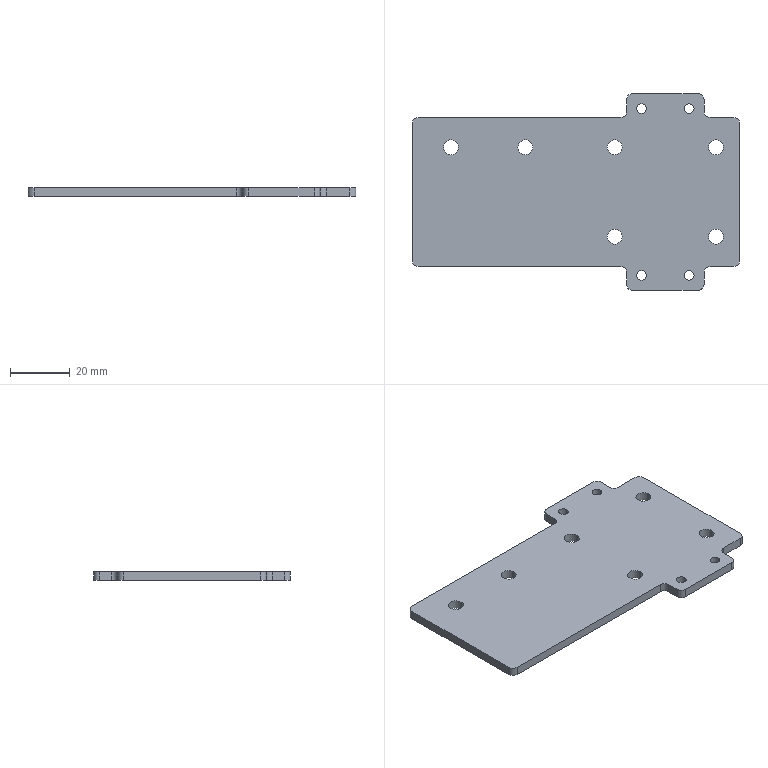Part | SolidWorks | features BaseBody 1 | 1 solid | 46 faces | box 110 x 66 x 3 mm | volume 17285 mm3 | cylinder 32 | plane 14 | commonest cylinder face diameters 4 x12 5 x12 3.24 x8
STEP:
#1=CARTESIAN_POINT('',(20.38,-28.,3.));
#2=VERTEX_POINT('',#1);
#3=CARTESIAN_POINT('',(23.62,-28.,3.));
#4=VERTEX_POINT('',#3);
#5=CARTESIAN_POINT('',(22.,-28.,3.));
#6=DIRECTION('',(0.,0.,1.));
#7=DIRECTION('',(-1.,0.,0.));
#8=AXIS2_PLACEMENT_3D('',#5,#6,#7);
#9=CIRCLE('',#8,1.62);
#10=EDGE_CURVE('',#2,#4,#9,.T.);
#11=ORIENTED_EDGE('',*,*,#10,.T.);
#12=CARTESIAN_POINT('',(23.62,-28.,0.));
#13=VERTEX_POINT('',#12);
#14=CARTESIAN_POINT('',(23.62,-28.,3.));
#15=DIRECTION('',(0.,0.,-1.));
#16=VECTOR('',#15,1000.);
#17=LINE('',#14,#16);
#18=EDGE_CURVE('',#4,#13,#17,.T.);
#19=ORIENTED_EDGE('',*,*,#18,.T.);
#20=CARTESIAN_POINT('',(20.38,-28.,0.));
#21=VERTEX_POINT('',#20);
#22=CARTESIAN_POINT('',(22.,-28.,0.));
#23=DIRECTION('',(0.,0.,1.));
#24=DIRECTION('',(-1.,0.,0.));
#25=AXIS2_PLACEMENT_3D('',#22,#23,#24);
#26=CIRCLE('',#25,1.62);
#27=EDGE_CURVE('',#21,#13,#26,.T.);
#28=ORIENTED_EDGE('',*,*,#27,.F.);
#29=CARTESIAN_POINT('',(20.38,-28.,3.));
#30=DIRECTION('',(0.,0.,-1.));
#31=VECTOR('',#30,1000.);
#32=LINE('',#29,#31);
#33=EDGE_CURVE('',#2,#21,#32,.T.);
#34=ORIENTED_EDGE('',*,*,#33,.F.);
#35=EDGE_LOOP('',(#11,#19,#28,#34));
#36=FACE_OUTER_BOUND('',#35,.T.);
#37=CARTESIAN_POINT('',(22.,-28.,3.));
#38=DIRECTION('',(0.,0.,-1.));
#39=DIRECTION('',(-1.,0.,0.));
#40=AXIS2_PLACEMENT_3D('',#37,#38,#39);
#41=CYLINDRICAL_SURFACE('',#40,1.62);
#42=ADVANCED_FACE('',(#36),#41,.F.);
#43=CARTESIAN_POINT('',(36.38,-28.,3.));
#44=VERTEX_POINT('',#43);
#45=CARTESIAN_POINT('',(39.62,-28.,3.));
#46=VERTEX_POINT('',#45);
#47=CARTESIAN_POINT('',(38.,-28.,3.));
#48=DIRECTION('',(0.,0.,1.));
#49=DIRECTION('',(-1.,0.,0.));
#50=AXIS2_PLACEMENT_3D('',#47,#48,#49);
#51=CIRCLE('',#50,1.62);
#52=EDGE_CURVE('',#44,#46,#51,.T.);
#53=ORIENTED_EDGE('',*,*,#52,.T.);
#54=CARTESIAN_POINT('',(39.62,-28.,0.));
#55=VERTEX_POINT('',#54);
#56=CARTESIAN_POINT('',(39.62,-28.,3.));
#57=DIRECTION('',(0.,0.,-1.));
#58=VECTOR('',#57,1000.);
#59=LINE('',#56,#58);
#60=EDGE_CURVE('',#46,#55,#59,.T.);
#61=ORIENTED_EDGE('',*,*,#60,.T.);
#62=CARTESIAN_POINT('',(36.38,-28.,0.));
#63=VERTEX_POINT('',#62);
#64=CARTESIAN_POINT('',(38.,-28.,0.));
#65=DIRECTION('',(0.,0.,1.));
#66=DIRECTION('',(-1.,0.,0.));
#67=AXIS2_PLACEMENT_3D('',#64,#65,#66);
#68=CIRCLE('',#67,1.62);
#69=EDGE_CURVE('',#63,#55,#68,.T.);
#70=ORIENTED_EDGE('',*,*,#69,.F.);
#71=CARTESIAN_POINT('',(36.38,-28.,3.));
#72=DIRECTION('',(0.,0.,-1.));
#73=VECTOR('',#72,1000.);
#74=LINE('',#71,#73);
#75=EDGE_CURVE('',#44,#63,#74,.T.);
#76=ORIENTED_EDGE('',*,*,#75,.F.);
#77=EDGE_LOOP('',(#53,#61,#70,#76));
#78=FACE_OUTER_BOUND('',#77,.T.);
#79=CARTESIAN_POINT('',(38.,-28.,3.));
#80=DIRECTION('',(0.,0.,-1.));
#81=DIRECTION('',(-1.,0.,0.));
#82=AXIS2_PLACEMENT_3D('',#79,#80,#81);
#83=CYLINDRICAL_SURFACE('',#82,1.62);
#84=ADVANCED_FACE('',(#78),#83,.F.);
#85=CARTESIAN_POINT('',(36.38,28.,3.));
#86=VERTEX_POINT('',#85);
#87=CARTESIAN_POINT('',(39.62,28.,3.));
#88=VERTEX_POINT('',#87);
#89=CARTESIAN_POINT('',(38.,28.,3.));
#90=DIRECTION('',(0.,0.,1.));
#91=DIRECTION('',(-1.,0.,0.));
#92=AXIS2_PLACEMENT_3D('',#89,#90,#91);
#93=CIRCLE('',#92,1.62);
#94=EDGE_CURVE('',#86,#88,#93,.T.);
#95=ORIENTED_EDGE('',*,*,#94,.T.);
#96=CARTESIAN_POINT('',(39.62,28.,0.));
#97=VERTEX_POINT('',#96);
#98=CARTESIAN_POINT('',(39.62,28.,3.));
#99=DIRECTION('',(0.,0.,-1.));
#100=VECTOR('',#99,1000.);
#101=LINE('',#98,#100);
#102=EDGE_CURVE('',#88,#97,#101,.T.);
#103=ORIENTED_EDGE('',*,*,#102,.T.);
#104=CARTESIAN_POINT('',(36.38,28.,0.));
#105=VERTEX_POINT('',#104);
#106=CARTESIAN_POINT('',(38.,28.,0.));
#107=DIRECTION('',(0.,0.,1.));
#108=DIRECTION('',(-1.,0.,0.));
#109=AXIS2_PLACEMENT_3D('',#106,#107,#108);
#110=CIRCLE('',#109,1.62);
#111=EDGE_CURVE('',#105,#97,#110,.T.);
#112=ORIENTED_EDGE('',*,*,#111,.F.);
#113=CARTESIAN_POINT('',(36.38,28.,3.));
#114=DIRECTION('',(0.,0.,-1.));
#115=VECTOR('',#114,1000.);
#116=LINE('',#113,#115);
#117=EDGE_CURVE('',#86,#105,#116,.T.);
#118=ORIENTED_EDGE('',*,*,#117,.F.);
#119=EDGE_LOOP('',(#95,#103,#112,#118));
#120=FACE_OUTER_BOUND('',#119,.T.);
#121=CARTESIAN_POINT('',(38.,28.,3.));
#122=DIRECTION('',(0.,0.,-1.));
#123=DIRECTION('',(-1.,0.,0.));
#124=AXIS2_PLACEMENT_3D('',#121,#122,#123);
#125=CYLINDRICAL_SURFACE('',#124,1.62);
#126=ADVANCED_FACE('',(#120),#125,.F.);
#127=CARTESIAN_POINT('',(20.38,28.,3.));
#128=VERTEX_POINT('',#127);
#129=CARTESIAN_POINT('',(23.62,28.,3.));
#130=VERTEX_POINT('',#129);
#131=CARTESIAN_POINT('',(22.,28.,3.));
#132=DIRECTION('',(0.,0.,1.));
#133=DIRECTION('',(-1.,0.,0.));
#134=AXIS2_PLACEMENT_3D('',#131,#132,#133);
#135=CIRCLE('',#134,1.62);
#136=EDGE_CURVE('',#128,#130,#135,.T.);
#137=ORIENTED_EDGE('',*,*,#136,.T.);
#138=CARTESIAN_POINT('',(23.62,28.,0.));
#139=VERTEX_POINT('',#138);
#140=CARTESIAN_POINT('',(23.62,28.,3.));
#141=DIRECTION('',(0.,0.,-1.));
#142=VECTOR('',#141,1000.);
#143=LINE('',#140,#142);
#144=EDGE_CURVE('',#130,#139,#143,.T.);
#145=ORIENTED_EDGE('',*,*,#144,.T.);
#146=CARTESIAN_POINT('',(20.38,28.,0.));
#147=VERTEX_POINT('',#146);
#148=CARTESIAN_POINT('',(22.,28.,0.));
#149=DIRECTION('',(0.,0.,1.));
#150=DIRECTION('',(-1.,0.,0.));
#151=AXIS2_PLACEMENT_3D('',#148,#149,#150);
#152=CIRCLE('',#151,1.62);
#153=EDGE_CURVE('',#147,#139,#152,.T.);
#154=ORIENTED_EDGE('',*,*,#153,.F.);
#155=CARTESIAN_POINT('',(20.38,28.,3.));
#156=DIRECTION('',(0.,0.,-1.));
#157=VECTOR('',#156,1000.);
#158=LINE('',#155,#157);
#159=EDGE_CURVE('',#128,#147,#158,.T.);
#160=ORIENTED_EDGE('',*,*,#159,.F.);
#161=EDGE_LOOP('',(#137,#145,#154,#160));
#162=FACE_OUTER_BOUND('',#161,.T.);
#163=CARTESIAN_POINT('',(22.,28.,3.));
#164=DIRECTION('',(0.,0.,-1.));
#165=DIRECTION('',(-1.,0.,0.));
#166=AXIS2_PLACEMENT_3D('',#163,#164,#165);
#167=CYLINDRICAL_SURFACE('',#166,1.62);
#168=ADVANCED_FACE('',(#162),#167,.F.);
#169=CARTESIAN_POINT('',(10.5,-15.,3.));
#170=VERTEX_POINT('',#169);
#171=CARTESIAN_POINT('',(15.5,-15.,3.));
#172=VERTEX_POINT('',#171);
#173=CARTESIAN_POINT('',(13.,-15.,3.));
#174=DIRECTION('',(0.,0.,1.));
#175=DIRECTION('',(-1.,0.,0.));
#176=AXIS2_PLACEMENT_3D('',#173,#174,#175);
#177=CIRCLE('',#176,2.5);
#178=EDGE_CURVE('',#170,#172,#177,.T.);
#179=ORIENTED_EDGE('',*,*,#178,.T.);
#180=CARTESIAN_POINT('',(15.5,-15.,0.));
#181=VERTEX_POINT('',#180);
#182=CARTESIAN_POINT('',(15.5,-15.,3.));
#183=DIRECTION('',(0.,0.,-1.));
#184=VECTOR('',#183,1000.);
#185=LINE('',#182,#184);
#186=EDGE_CURVE('',#172,#181,#185,.T.);
#187=ORIENTED_EDGE('',*,*,#186,.T.);
#188=CARTESIAN_POINT('',(10.5,-15.,0.));
#189=VERTEX_POINT('',#188);
#190=CARTESIAN_POINT('',(13.,-15.,0.));
#191=DIRECTION('',(0.,0.,1.));
#192=DIRECTION('',(-1.,0.,0.));
#193=AXIS2_PLACEMENT_3D('',#190,#191,#192);
#194=CIRCLE('',#193,2.5);
#195=EDGE_CURVE('',#189,#181,#194,.T.);
#196=ORIENTED_EDGE('',*,*,#195,.F.);
#197=CARTESIAN_POINT('',(10.5,-15.,3.));
#198=DIRECTION('',(0.,0.,-1.));
#199=VECTOR('',#198,1000.);
#200=LINE('',#197,#199);
#201=EDGE_CURVE('',#170,#189,#200,.T.);
#202=ORIENTED_EDGE('',*,*,#201,.F.);
#203=EDGE_LOOP('',(#179,#187,#196,#202));
#204=FACE_OUTER_BOUND('',#203,.T.);
#205=CARTESIAN_POINT('',(13.,-15.,3.));
#206=DIRECTION('',(0.,0.,-1.));
#207=DIRECTION('',(-1.,0.,0.));
#208=AXIS2_PLACEMENT_3D('',#205,#206,#207);
#209=CYLINDRICAL_SURFACE('',#208,2.5);
#210=ADVANCED_FACE('',(#204),#209,.F.);
#211=CARTESIAN_POINT('',(10.5,15.,3.));
#212=VERTEX_POINT('',#211);
#213=CARTESIAN_POINT('',(15.5,15.,3.));
#214=VERTEX_POINT('',#213);
#215=CARTESIAN_POINT('',(13.,15.,3.));
#216=DIRECTION('',(0.,0.,1.));
#217=DIRECTION('',(-1.,0.,0.));
#218=AXIS2_PLACEMENT_3D('',#215,#216,#217);
#219=CIRCLE('',#218,2.5);
#220=EDGE_CURVE('',#212,#214,#219,.T.);
#221=ORIENTED_EDGE('',*,*,#220,.T.);
#222=CARTESIAN_POINT('',(15.5,15.,0.));
#223=VERTEX_POINT('',#222);
#224=CARTESIAN_POINT('',(15.5,15.,3.));
#225=DIRECTION('',(0.,0.,-1.));
#226=VECTOR('',#225,1000.);
#227=LINE('',#224,#226);
#228=EDGE_CURVE('',#214,#223,#227,.T.);
#229=ORIENTED_EDGE('',*,*,#228,.T.);
#230=CARTESIAN_POINT('',(10.5,15.,0.));
#231=VERTEX_POINT('',#230);
#232=CARTESIAN_POINT('',(13.,15.,0.));
#233=DIRECTION('',(0.,0.,1.));
#234=DIRECTION('',(-1.,0.,0.));
#235=AXIS2_PLACEMENT_3D('',#232,#233,#234);
#236=CIRCLE('',#235,2.5);
#237=EDGE_CURVE('',#231,#223,#236,.T.);
#238=ORIENTED_EDGE('',*,*,#237,.F.);
#239=CARTESIAN_POINT('',(10.5,15.,3.));
#240=DIRECTION('',(0.,0.,-1.));
#241=VECTOR('',#240,1000.);
#242=LINE('',#239,#241);
#243=EDGE_CURVE('',#212,#231,#242,.T.);
#244=ORIENTED_EDGE('',*,*,#243,.F.);
#245=EDGE_LOOP('',(#221,#229,#238,#244));
#246=FACE_OUTER_BOUND('',#245,.T.);
#247=CARTESIAN_POINT('',(13.,15.,3.));
#248=DIRECTION('',(0.,0.,-1.));
#249=DIRECTION('',(-1.,0.,0.));
#250=AXIS2_PLACEMENT_3D('',#247,#248,#249);
#251=CYLINDRICAL_SURFACE('',#250,2.5);
#252=ADVANCED_FACE('',(#246),#251,.F.);
#253=CARTESIAN_POINT('',(-44.5,15.,3.));
#254=VERTEX_POINT('',#253);
#255=CARTESIAN_POINT('',(-39.5,15.,3.));
#256=VERTEX_POINT('',#255);
#257=CARTESIAN_POINT('',(-42.,15.,3.));
#258=DIRECTION('',(0.,0.,1.));
#259=DIRECTION('',(-1.,0.,0.));
#260=AXIS2_PLACEMENT_3D('',#257,#258,#259);
#261=CIRCLE('',#260,2.5);
#262=EDGE_CURVE('',#254,#256,#261,.T.);
#263=ORIENTED_EDGE('',*,*,#262,.T.);
#264=CARTESIAN_POINT('',(-39.5,15.,0.));
#265=VERTEX_POINT('',#264);
#266=CARTESIAN_POINT('',(-39.5,15.,3.));
#267=DIRECTION('',(0.,0.,-1.));
#268=VECTOR('',#267,1000.);
#269=LINE('',#266,#268);
#270=EDGE_CURVE('',#256,#265,#269,.T.);
#271=ORIENTED_EDGE('',*,*,#270,.T.);
#272=CARTESIAN_POINT('',(-44.5,15.,0.));
#273=VERTEX_POINT('',#272);
#274=CARTESIAN_POINT('',(-42.,15.,0.));
#275=DIRECTION('',(0.,0.,1.));
#276=DIRECTION('',(-1.,0.,0.));
#277=AXIS2_PLACEMENT_3D('',#274,#275,#276);
#278=CIRCLE('',#277,2.5);
#279=EDGE_CURVE('',#273,#265,#278,.T.);
#280=ORIENTED_EDGE('',*,*,#279,.F.);
#281=CARTESIAN_POINT('',(-44.5,15.,3.));
#282=DIRECTION('',(0.,0.,-1.));
#283=VECTOR('',#282,1000.);
#284=LINE('',#281,#283);
#285=EDGE_CURVE('',#254,#273,#284,.T.);
#286=ORIENTED_EDGE('',*,*,#285,.F.);
#287=EDGE_LOOP('',(#263,#271,#280,#286));
#288=FACE_OUTER_BOUND('',#287,.T.);
#289=CARTESIAN_POINT('',(-42.,15.,3.));
#290=DIRECTION('',(0.,0.,-1.));
#291=DIRECTION('',(-1.,0.,0.));
#292=AXIS2_PLACEMENT_3D('',#289,#290,#291);
#293=CYLINDRICAL_SURFACE('',#292,2.5);
#294=ADVANCED_FACE('',(#288),#293,.F.);
#295=CARTESIAN_POINT('',(-19.5,15.,3.));
#296=VERTEX_POINT('',#295);
#297=CARTESIAN_POINT('',(-14.5,15.,3.));
#298=VERTEX_POINT('',#297);
#299=CARTESIAN_POINT('',(-17.,15.,3.));
#300=DIRECTION('',(0.,0.,1.));
#301=DIRECTION('',(-1.,0.,0.));
#302=AXIS2_PLACEMENT_3D('',#299,#300,#301);
#303=CIRCLE('',#302,2.5);
#304=EDGE_CURVE('',#296,#298,#303,.T.);
#305=ORIENTED_EDGE('',*,*,#304,.T.);
#306=CARTESIAN_POINT('',(-14.5,15.,0.));
#307=VERTEX_POINT('',#306);
#308=CARTESIAN_POINT('',(-14.5,15.,3.));
#309=DIRECTION('',(0.,0.,-1.));
#310=VECTOR('',#309,1000.);
#311=LINE('',#308,#310);
#312=EDGE_CURVE('',#298,#307,#311,.T.);
#313=ORIENTED_EDGE('',*,*,#312,.T.);
#314=CARTESIAN_POINT('',(-19.5,15.,0.));
#315=VERTEX_POINT('',#314);
#316=CARTESIAN_POINT('',(-17.,15.,0.));
#317=DIRECTION('',(0.,0.,1.));
#318=DIRECTION('',(-1.,0.,0.));
#319=AXIS2_PLACEMENT_3D('',#316,#317,#318);
#320=CIRCLE('',#319,2.5);
#321=EDGE_CURVE('',#315,#307,#320,.T.);
#322=ORIENTED_EDGE('',*,*,#321,.F.);
#323=CARTESIAN_POINT('',(-19.5,15.,3.));
#324=DIRECTION('',(0.,0.,-1.));
#325=VECTOR('',#324,1000.);
#326=LINE('',#323,#325);
#327=EDGE_CURVE('',#296,#315,#326,.T.);
#328=ORIENTED_EDGE('',*,*,#327,.F.);
#329=EDGE_LOOP('',(#305,#313,#322,#328));
#330=FACE_OUTER_BOUND('',#329,.T.);
#331=CARTESIAN_POINT('',(-17.,15.,3.));
#332=DIRECTION('',(0.,0.,-1.));
#333=DIRECTION('',(-1.,0.,0.));
#334=AXIS2_PLACEMENT_3D('',#331,#332,#333);
#335=CYLINDRICAL_SURFACE('',#334,2.5);
#336=ADVANCED_FACE('',(#330),#335,.F.);
#337=CARTESIAN_POINT('',(44.5,-15.,3.));
#338=VERTEX_POINT('',#337);
#339=CARTESIAN_POINT('',(49.5,-15.,3.));
#340=VERTEX_POINT('',#339);
#341=CARTESIAN_POINT('',(47.,-15.,3.));
#342=DIRECTION('',(0.,0.,1.));
#343=DIRECTION('',(-1.,0.,0.));
#344=AXIS2_PLACEMENT_3D('',#341,#342,#343);
#345=CIRCLE('',#344,2.5);
#346=EDGE_CURVE('',#338,#340,#345,.T.);
#347=ORIENTED_EDGE('',*,*,#346,.T.);
#348=CARTESIAN_POINT('',(49.5,-15.,0.));
#349=VERTEX_POINT('',#348);
#350=CARTESIAN_POINT('',(49.5,-15.,3.));
#351=DIRECTION('',(0.,0.,-1.));
#352=VECTOR('',#351,1000.);
#353=LINE('',#350,#352);
#354=EDGE_CURVE('',#340,#349,#353,.T.);
#355=ORIENTED_EDGE('',*,*,#354,.T.);
#356=CARTESIAN_POINT('',(44.5,-15.,0.));
#357=VERTEX_POINT('',#356);
#358=CARTESIAN_POINT('',(47.,-15.,0.));
#359=DIRECTION('',(0.,0.,1.));
#360=DIRECTION('',(-1.,0.,0.));
#361=AXIS2_PLACEMENT_3D('',#358,#359,#360);
#362=CIRCLE('',#361,2.5);
#363=EDGE_CURVE('',#357,#349,#362,.T.);
#364=ORIENTED_EDGE('',*,*,#363,.F.);
#365=CARTESIAN_POINT('',(44.5,-15.,3.));
#366=DIRECTION('',(0.,0.,-1.));
#367=VECTOR('',#366,1000.);
#368=LINE('',#365,#367);
#369=EDGE_CURVE('',#338,#357,#368,.T.);
#370=ORIENTED_EDGE('',*,*,#369,.F.);
#371=EDGE_LOOP('',(#347,#355,#364,#370));
#372=FACE_OUTER_BOUND('',#371,.T.);
#373=CARTESIAN_POINT('',(47.,-15.,3.));
#374=DIRECTION('',(0.,0.,-1.));
#375=DIRECTION('',(-1.,0.,0.));
#376=AXIS2_PLACEMENT_3D('',#373,#374,#375);
#377=CYLINDRICAL_SURFACE('',#376,2.5);
#378=ADVANCED_FACE('',(#372),#377,.F.);
#379=CARTESIAN_POINT('',(44.5,15.,3.));
#380=VERTEX_POINT('',#379);
#381=CARTESIAN_POINT('',(49.5,15.,3.));
#382=VERTEX_POINT('',#381);
#383=CARTESIAN_POINT('',(47.,15.,3.));
#384=DIRECTION('',(0.,0.,1.));
#385=DIRECTION('',(-1.,0.,0.));
#386=AXIS2_PLACEMENT_3D('',#383,#384,#385);
#387=CIRCLE('',#386,2.5);
#388=EDGE_CURVE('',#380,#382,#387,.T.);
#389=ORIENTED_EDGE('',*,*,#388,.T.);
#390=CARTESIAN_POINT('',(49.5,15.,0.));
#391=VERTEX_POINT('',#390);
#392=CARTESIAN_POINT('',(49.5,15.,3.));
#393=DIRECTION('',(0.,0.,-1.));
#394=VECTOR('',#393,1000.);
#395=LINE('',#392,#394);
#396=EDGE_CURVE('',#382,#391,#395,.T.);
#397=ORIENTED_EDGE('',*,*,#396,.T.);
#398=CARTESIAN_POINT('',(44.5,15.,0.));
#399=VERTEX_POINT('',#398);
#400=CARTESIAN_POINT('',(47.,15.,0.));
#401=DIRECTION('',(0.,0.,1.));
#402=DIRECTION('',(-1.,0.,0.));
#403=AXIS2_PLACEMENT_3D('',#400,#401,#402);
#404=CIRCLE('',#403,2.5);
#405=EDGE_CURVE('',#399,#391,#404,.T.);
#406=ORIENTED_EDGE('',*,*,#405,.F.);
#407=CARTESIAN_POINT('',(44.5,15.,3.));
#408=DIRECTION('',(0.,0.,-1.));
#409=VECTOR('',#408,1000.);
#410=LINE('',#407,#409);
#411=EDGE_CURVE('',#380,#399,#410,.T.);
#412=ORIENTED_EDGE('',*,*,#411,.F.);
#413=EDGE_LOOP('',(#389,#397,#406,#412));
#414=FACE_OUTER_BOUND('',#413,.T.);
#415=CARTESIAN_POINT('',(47.,15.,3.));
#416=DIRECTION('',(0.,0.,-1.));
#417=DIRECTION('',(-1.,0.,0.));
#418=AXIS2_PLACEMENT_3D('',#415,#416,#417);
#419=CYLINDRICAL_SURFACE('',#418,2.5);
#420=ADVANCED_FACE('',(#414),#419,.F.);
#421=ORIENTED_EDGE('',*,*,#10,.F.);
#422=CARTESIAN_POINT('',(22.,-28.,3.));
#423=DIRECTION('',(0.,0.,1.));
#424=DIRECTION('',(-1.,0.,0.));
#425=AXIS2_PLACEMENT_3D('',#422,#423,#424);
#426=CIRCLE('',#425,1.62);
#427=EDGE_CURVE('',#4,#2,#426,.T.);
#428=ORIENTED_EDGE('',*,*,#427,.F.);
#429=EDGE_LOOP('',(#421,#428));
#430=FACE_BOUND('',#429,.T.);
#431=ORIENTED_EDGE('',*,*,#52,.F.);
#432=CARTESIAN_POINT('',(38.,-28.,3.));
#433=DIRECTION('',(0.,0.,1.));
#434=DIRECTION('',(-1.,0.,0.));
#435=AXIS2_PLACEMENT_3D('',#432,#433,#434);
#436=CIRCLE('',#435,1.62);
#437=EDGE_CURVE('',#46,#44,#436,.T.);
#438=ORIENTED_EDGE('',*,*,#437,.F.);
#439=EDGE_LOOP('',(#431,#438));
#440=FACE_BOUND('',#439,.T.);
#441=ORIENTED_EDGE('',*,*,#94,.F.);
#442=CARTESIAN_POINT('',(38.,28.,3.));
#443=DIRECTION('',(0.,0.,1.));
#444=DIRECTION('',(-1.,0.,0.));
#445=AXIS2_PLACEMENT_3D('',#442,#443,#444);
#446=CIRCLE('',#445,1.62);
#447=EDGE_CURVE('',#88,#86,#446,.T.);
#448=ORIENTED_EDGE('',*,*,#447,.F.);
#449=EDGE_LOOP('',(#441,#448));
#450=FACE_BOUND('',#449,.T.);
#451=ORIENTED_EDGE('',*,*,#136,.F.);
#452=CARTESIAN_POINT('',(22.,28.,3.));
#453=DIRECTION('',(0.,0.,1.));
#454=DIRECTION('',(-1.,0.,0.));
#455=AXIS2_PLACEMENT_3D('',#452,#453,#454);
#456=CIRCLE('',#455,1.62);
#457=EDGE_CURVE('',#130,#128,#456,.T.);
#458=ORIENTED_EDGE('',*,*,#457,.F.);
#459=EDGE_LOOP('',(#451,#458));
#460=FACE_BOUND('',#459,.T.);
#461=ORIENTED_EDGE('',*,*,#178,.F.);
#462=CARTESIAN_POINT('',(13.,-15.,3.));
#463=DIRECTION('',(0.,0.,1.));
#464=DIRECTION('',(-1.,0.,0.));
#465=AXIS2_PLACEMENT_3D('',#462,#463,#464);
#466=CIRCLE('',#465,2.5);
#467=EDGE_CURVE('',#172,#170,#466,.T.);
#468=ORIENTED_EDGE('',*,*,#467,.F.);
#469=EDGE_LOOP('',(#461,#468));
#470=FACE_BOUND('',#469,.T.);
#471=ORIENTED_EDGE('',*,*,#220,.F.);
#472=CARTESIAN_POINT('',(13.,15.,3.));
#473=DIRECTION('',(0.,0.,1.));
#474=DIRECTION('',(-1.,0.,0.));
#475=AXIS2_PLACEMENT_3D('',#472,#473,#474);
#476=CIRCLE('',#475,2.5);
#477=EDGE_CURVE('',#214,#212,#476,.T.);
#478=ORIENTED_EDGE('',*,*,#477,.F.);
#479=EDGE_LOOP('',(#471,#478));
#480=FACE_BOUND('',#479,.T.);
#481=ORIENTED_EDGE('',*,*,#262,.F.);
#482=CARTESIAN_POINT('',(-42.,15.,3.));
#483=DIRECTION('',(0.,0.,1.));
#484=DIRECTION('',(-1.,0.,0.));
#485=AXIS2_PLACEMENT_3D('',#482,#483,#484);
#486=CIRCLE('',#485,2.5);
#487=EDGE_CURVE('',#256,#254,#486,.T.);
#488=ORIENTED_EDGE('',*,*,#487,.F.);
#489=EDGE_LOOP('',(#481,#488));
#490=FACE_BOUND('',#489,.T.);
#491=ORIENTED_EDGE('',*,*,#304,.F.);
#492=CARTESIAN_POINT('',(-17.,15.,3.));
#493=DIRECTION('',(0.,0.,1.));
#494=DIRECTION('',(-1.,0.,0.));
#495=AXIS2_PLACEMENT_3D('',#492,#493,#494);
#496=CIRCLE('',#495,2.5);
#497=EDGE_CURVE('',#298,#296,#496,.T.);
#498=ORIENTED_EDGE('',*,*,#497,.F.);
#499=EDGE_LOOP('',(#491,#498));
#500=FACE_BOUND('',#499,.T.);
#501=ORIENTED_EDGE('',*,*,#346,.F.);
#502=CARTESIAN_POINT('',(47.,-15.,3.));
#503=DIRECTION('',(0.,0.,1.));
#504=DIRECTION('',(-1.,0.,0.));
#505=AXIS2_PLACEMENT_3D('',#502,#503,#504);
#506=CIRCLE('',#505,2.5);
#507=EDGE_CURVE('',#340,#338,#506,.T.);
#508=ORIENTED_EDGE('',*,*,#507,.F.);
#509=EDGE_LOOP('',(#501,#508));
#510=FACE_BOUND('',#509,.T.);
#511=ORIENTED_EDGE('',*,*,#388,.F.);
#512=CARTESIAN_POINT('',(47.,15.,3.));
#513=DIRECTION('',(0.,0.,1.));
#514=DIRECTION('',(-1.,0.,0.));
#515=AXIS2_PLACEMENT_3D('',#512,#513,#514);
#516=CIRCLE('',#515,2.5);
#517=EDGE_CURVE('',#382,#380,#516,.T.);
#518=ORIENTED_EDGE('',*,*,#517,.F.);
#519=EDGE_LOOP('',(#511,#518));
#520=FACE_BOUND('',#519,.T.);
#521=CARTESIAN_POINT('',(19.,-33.,3.));
#522=VERTEX_POINT('',#521);
#523=CARTESIAN_POINT('',(17.,-31.,3.));
#524=VERTEX_POINT('',#523);
#525=CARTESIAN_POINT('',(19.,-31.,3.));
#526=DIRECTION('',(0.,0.,-1.));
#527=DIRECTION('',(-1.,0.,0.));
#528=AXIS2_PLACEMENT_3D('',#525,#526,#527);
#529=CIRCLE('',#528,2.);
#530=EDGE_CURVE('',#522,#524,#529,.T.);
#531=ORIENTED_EDGE('',*,*,#530,.F.);
#532=CARTESIAN_POINT('',(41.,-33.,3.));
#533=VERTEX_POINT('',#532);
#534=CARTESIAN_POINT('',(0.,-33.,3.));
#535=DIRECTION('',(-1.,0.,0.));
#536=VECTOR('',#535,1000.);
#537=LINE('',#534,#536);
#538=EDGE_CURVE('',#533,#522,#537,.T.);
#539=ORIENTED_EDGE('',*,*,#538,.F.);
#540=CARTESIAN_POINT('',(43.,-31.,3.));
#541=VERTEX_POINT('',#540);
#542=CARTESIAN_POINT('',(41.,-31.,3.));
#543=DIRECTION('',(0.,0.,-1.));
#544=DIRECTION('',(-1.,0.,0.));
#545=AXIS2_PLACEMENT_3D('',#542,#543,#544);
#546=CIRCLE('',#545,2.);
#547=EDGE_CURVE('',#541,#533,#546,.T.);
#548=ORIENTED_EDGE('',*,*,#547,.F.);
#549=CARTESIAN_POINT('',(43.,-27.,3.));
#550=VERTEX_POINT('',#549);
#551=CARTESIAN_POINT('',(43.,0.,3.));
#552=DIRECTION('',(0.,-1.,0.));
#553=VECTOR('',#552,1000.);
#554=LINE('',#551,#553);
#555=EDGE_CURVE('',#550,#541,#554,.T.);
#556=ORIENTED_EDGE('',*,*,#555,.F.);
#557=CARTESIAN_POINT('',(45.,-25.,3.));
#558=VERTEX_POINT('',#557);
#559=CARTESIAN_POINT('',(45.,-27.,3.));
#560=DIRECTION('',(0.,0.,1.));
#561=DIRECTION('',(-1.,0.,0.));
#562=AXIS2_PLACEMENT_3D('',#559,#560,#561);
#563=CIRCLE('',#562,2.);
#564=EDGE_CURVE('',#558,#550,#563,.T.);
#565=ORIENTED_EDGE('',*,*,#564,.F.);
#566=CARTESIAN_POINT('',(53.,-25.,3.));
#567=VERTEX_POINT('',#566);
#568=CARTESIAN_POINT('',(0.,-25.,3.));
#569=DIRECTION('',(-1.,0.,0.));
#570=VECTOR('',#569,1000.);
#571=LINE('',#568,#570);
#572=EDGE_CURVE('',#567,#558,#571,.T.);
#573=ORIENTED_EDGE('',*,*,#572,.F.);
#574=CARTESIAN_POINT('',(55.,-23.,3.));
#575=VERTEX_POINT('',#574);
#576=CARTESIAN_POINT('',(53.,-23.,3.));
#577=DIRECTION('',(0.,0.,-1.));
#578=DIRECTION('',(-1.,0.,0.));
#579=AXIS2_PLACEMENT_3D('',#576,#577,#578);
#580=CIRCLE('',#579,2.);
#581=EDGE_CURVE('',#575,#567,#580,.T.);
#582=ORIENTED_EDGE('',*,*,#581,.F.);
#583=CARTESIAN_POINT('',(55.,23.,3.));
#584=VERTEX_POINT('',#583);
#585=CARTESIAN_POINT('',(55.,0.,3.));
#586=DIRECTION('',(0.,-1.,0.));
#587=VECTOR('',#586,1000.);
#588=LINE('',#585,#587);
#589=EDGE_CURVE('',#584,#575,#588,.T.);
#590=ORIENTED_EDGE('',*,*,#589,.F.);
#591=CARTESIAN_POINT('',(53.,25.,3.));
#592=VERTEX_POINT('',#591);
#593=CARTESIAN_POINT('',(53.,23.,3.));
#594=DIRECTION('',(0.,0.,-1.));
#595=DIRECTION('',(-1.,0.,0.));
#596=AXIS2_PLACEMENT_3D('',#593,#594,#595);
#597=CIRCLE('',#596,2.);
#598=EDGE_CURVE('',#592,#584,#597,.T.);
#599=ORIENTED_EDGE('',*,*,#598,.F.);
#600=CARTESIAN_POINT('',(45.,25.,3.));
#601=VERTEX_POINT('',#600);
#602=CARTESIAN_POINT('',(0.,25.,3.));
#603=DIRECTION('',(1.,0.,0.));
#604=VECTOR('',#603,1000.);
#605=LINE('',#602,#604);
#606=EDGE_CURVE('',#601,#592,#605,.T.);
#607=ORIENTED_EDGE('',*,*,#606,.F.);
#608=CARTESIAN_POINT('',(43.,27.,3.));
#609=VERTEX_POINT('',#608);
#610=CARTESIAN_POINT('',(45.,27.,3.));
#611=DIRECTION('',(0.,0.,1.));
#612=DIRECTION('',(-1.,0.,0.));
#613=AXIS2_PLACEMENT_3D('',#610,#611,#612);
#614=CIRCLE('',#613,2.);
#615=EDGE_CURVE('',#609,#601,#614,.T.);
#616=ORIENTED_EDGE('',*,*,#615,.F.);
#617=CARTESIAN_POINT('',(43.,31.,3.));
#618=VERTEX_POINT('',#617);
#619=CARTESIAN_POINT('',(43.,0.,3.));
#620=DIRECTION('',(0.,-1.,0.));
#621=VECTOR('',#620,1000.);
#622=LINE('',#619,#621);
#623=EDGE_CURVE('',#618,#609,#622,.T.);
#624=ORIENTED_EDGE('',*,*,#623,.F.);
#625=CARTESIAN_POINT('',(41.,33.,3.));
#626=VERTEX_POINT('',#625);
#627=CARTESIAN_POINT('',(41.,31.,3.));
#628=DIRECTION('',(0.,0.,-1.));
#629=DIRECTION('',(-1.,0.,0.));
#630=AXIS2_PLACEMENT_3D('',#627,#628,#629);
#631=CIRCLE('',#630,2.);
#632=EDGE_CURVE('',#626,#618,#631,.T.);
#633=ORIENTED_EDGE('',*,*,#632,.F.);
#634=CARTESIAN_POINT('',(19.,33.,3.));
#635=VERTEX_POINT('',#634);
#636=CARTESIAN_POINT('',(0.,33.,3.));
#637=DIRECTION('',(1.,0.,0.));
#638=VECTOR('',#637,1000.);
#639=LINE('',#636,#638);
#640=EDGE_CURVE('',#635,#626,#639,.T.);
#641=ORIENTED_EDGE('',*,*,#640,.F.);
#642=CARTESIAN_POINT('',(17.,31.,3.));
#643=VERTEX_POINT('',#642);
#644=CARTESIAN_POINT('',(19.,31.,3.));
#645=DIRECTION('',(0.,0.,-1.));
#646=DIRECTION('',(-1.,0.,0.));
#647=AXIS2_PLACEMENT_3D('',#644,#645,#646);
#648=CIRCLE('',#647,2.);
#649=EDGE_CURVE('',#643,#635,#648,.T.);
#650=ORIENTED_EDGE('',*,*,#649,.F.);
#651=CARTESIAN_POINT('',(17.,27.,3.));
#652=VERTEX_POINT('',#651);
#653=CARTESIAN_POINT('',(17.,0.,3.));
#654=DIRECTION('',(0.,1.,0.));
#655=VECTOR('',#654,1000.);
#656=LINE('',#653,#655);
#657=EDGE_CURVE('',#652,#643,#656,.T.);
#658=ORIENTED_EDGE('',*,*,#657,.F.);
#659=CARTESIAN_POINT('',(15.,25.,3.));
#660=VERTEX_POINT('',#659);
#661=CARTESIAN_POINT('',(15.,27.,3.));
#662=DIRECTION('',(0.,0.,1.));
#663=DIRECTION('',(-1.,0.,0.));
#664=AXIS2_PLACEMENT_3D('',#661,#662,#663);
#665=CIRCLE('',#664,2.);
#666=EDGE_CURVE('',#660,#652,#665,.T.);
#667=ORIENTED_EDGE('',*,*,#666,.F.);
#668=CARTESIAN_POINT('',(-53.,25.,3.));
#669=VERTEX_POINT('',#668);
#670=CARTESIAN_POINT('',(0.,25.,3.));
#671=DIRECTION('',(1.,0.,0.));
#672=VECTOR('',#671,1000.);
#673=LINE('',#670,#672);
#674=EDGE_CURVE('',#669,#660,#673,.T.);
#675=ORIENTED_EDGE('',*,*,#674,.F.);
#676=CARTESIAN_POINT('',(-55.,23.,3.));
#677=VERTEX_POINT('',#676);
#678=CARTESIAN_POINT('',(-53.,23.,3.));
#679=DIRECTION('',(0.,0.,-1.));
#680=DIRECTION('',(-1.,0.,0.));
#681=AXIS2_PLACEMENT_3D('',#678,#679,#680);
#682=CIRCLE('',#681,2.);
#683=EDGE_CURVE('',#677,#669,#682,.T.);
#684=ORIENTED_EDGE('',*,*,#683,.F.);
#685=CARTESIAN_POINT('',(-55.,-23.,3.));
#686=VERTEX_POINT('',#685);
#687=CARTESIAN_POINT('',(-55.,0.,3.));
#688=DIRECTION('',(0.,1.,0.));
#689=VECTOR('',#688,1000.);
#690=LINE('',#687,#689);
#691=EDGE_CURVE('',#686,#677,#690,.T.);
#692=ORIENTED_EDGE('',*,*,#691,.F.);
#693=CARTESIAN_POINT('',(-53.,-25.,3.));
#694=VERTEX_POINT('',#693);
#695=CARTESIAN_POINT('',(-53.,-23.,3.));
#696=DIRECTION('',(0.,0.,-1.));
#697=DIRECTION('',(-1.,0.,0.));
#698=AXIS2_PLACEMENT_3D('',#695,#696,#697);
#699=CIRCLE('',#698,2.);
#700=EDGE_CURVE('',#694,#686,#699,.T.);
#701=ORIENTED_EDGE('',*,*,#700,.F.);
#702=CARTESIAN_POINT('',(15.,-25.,3.));
#703=VERTEX_POINT('',#702);
#704=CARTESIAN_POINT('',(0.,-25.,3.));
#705=DIRECTION('',(-1.,0.,0.));
#706=VECTOR('',#705,1000.);
#707=LINE('',#704,#706);
#708=EDGE_CURVE('',#703,#694,#707,.T.);
#709=ORIENTED_EDGE('',*,*,#708,.F.);
#710=CARTESIAN_POINT('',(17.,-27.,3.));
#711=VERTEX_POINT('',#710);
#712=CARTESIAN_POINT('',(15.,-27.,3.));
#713=DIRECTION('',(0.,0.,1.));
#714=DIRECTION('',(-1.,0.,0.));
#715=AXIS2_PLACEMENT_3D('',#712,#713,#714);
#716=CIRCLE('',#715,2.);
#717=EDGE_CURVE('',#711,#703,#716,.T.);
#718=ORIENTED_EDGE('',*,*,#717,.F.);
#719=CARTESIAN_POINT('',(17.,0.,3.));
#720=DIRECTION('',(0.,1.,0.));
#721=VECTOR('',#720,1000.);
#722=LINE('',#719,#721);
#723=EDGE_CURVE('',#524,#711,#722,.T.);
#724=ORIENTED_EDGE('',*,*,#723,.F.);
#725=EDGE_LOOP('',(#531,#539,#548,#556,#565,#573,#582,#590,#599,#607,#616,#624,#633,#641,#650,#658,#667,#675,#684,#692,#701,#709,#718,#724));
#726=FACE_OUTER_BOUND('',#725,.T.);
#727=CARTESIAN_POINT('',(0.,0.,3.));
#728=DIRECTION('',(0.,0.,-1.));
#729=DIRECTION('',(-1.,0.,0.));
#730=AXIS2_PLACEMENT_3D('',#727,#728,#729);
#731=PLANE('',#730);
#732=ADVANCED_FACE('',(#430,#440,#450,#460,#470,#480,#490,#500,#510,#520,#726),#731,.F.);
#733=ORIENTED_EDGE('',*,*,#18,.F.);
#734=ORIENTED_EDGE('',*,*,#427,.T.);
#735=ORIENTED_EDGE('',*,*,#33,.T.);
#736=CARTESIAN_POINT('',(22.,-28.,0.));
#737=DIRECTION('',(0.,0.,1.));
#738=DIRECTION('',(-1.,0.,0.));
#739=AXIS2_PLACEMENT_3D('',#736,#737,#738);
#740=CIRCLE('',#739,1.62);
#741=EDGE_CURVE('',#13,#21,#740,.T.);
#742=ORIENTED_EDGE('',*,*,#741,.F.);
#743=EDGE_LOOP('',(#733,#734,#735,#742));
#744=FACE_OUTER_BOUND('',#743,.T.);
#745=CARTESIAN_POINT('',(22.,-28.,3.));
#746=DIRECTION('',(0.,0.,-1.));
#747=DIRECTION('',(-1.,0.,0.));
#748=AXIS2_PLACEMENT_3D('',#745,#746,#747);
#749=CYLINDRICAL_SURFACE('',#748,1.62);
#750=ADVANCED_FACE('',(#744),#749,.F.);
#751=ORIENTED_EDGE('',*,*,#60,.F.);
#752=ORIENTED_EDGE('',*,*,#437,.T.);
#753=ORIENTED_EDGE('',*,*,#75,.T.);
#754=CARTESIAN_POINT('',(38.,-28.,0.));
#755=DIRECTION('',(0.,0.,1.));
#756=DIRECTION('',(-1.,0.,0.));
#757=AXIS2_PLACEMENT_3D('',#754,#755,#756);
#758=CIRCLE('',#757,1.62);
#759=EDGE_CURVE('',#55,#63,#758,.T.);
#760=ORIENTED_EDGE('',*,*,#759,.F.);
#761=EDGE_LOOP('',(#751,#752,#753,#760));
#762=FACE_OUTER_BOUND('',#761,.T.);
#763=CARTESIAN_POINT('',(38.,-28.,3.));
#764=DIRECTION('',(0.,0.,-1.));
#765=DIRECTION('',(-1.,0.,0.));
#766=AXIS2_PLACEMENT_3D('',#763,#764,#765);
#767=CYLINDRICAL_SURFACE('',#766,1.62);
#768=ADVANCED_FACE('',(#762),#767,.F.);
#769=ORIENTED_EDGE('',*,*,#102,.F.);
#770=ORIENTED_EDGE('',*,*,#447,.T.);
#771=ORIENTED_EDGE('',*,*,#117,.T.);
#772=CARTESIAN_POINT('',(38.,28.,0.));
#773=DIRECTION('',(0.,0.,1.));
#774=DIRECTION('',(-1.,0.,0.));
#775=AXIS2_PLACEMENT_3D('',#772,#773,#774);
#776=CIRCLE('',#775,1.62);
#777=EDGE_CURVE('',#97,#105,#776,.T.);
#778=ORIENTED_EDGE('',*,*,#777,.F.);
#779=EDGE_LOOP('',(#769,#770,#771,#778));
#780=FACE_OUTER_BOUND('',#779,.T.);
#781=CARTESIAN_POINT('',(38.,28.,3.));
#782=DIRECTION('',(0.,0.,-1.));
#783=DIRECTION('',(-1.,0.,0.));
#784=AXIS2_PLACEMENT_3D('',#781,#782,#783);
#785=CYLINDRICAL_SURFACE('',#784,1.62);
#786=ADVANCED_FACE('',(#780),#785,.F.);
#787=ORIENTED_EDGE('',*,*,#144,.F.);
#788=ORIENTED_EDGE('',*,*,#457,.T.);
#789=ORIENTED_EDGE('',*,*,#159,.T.);
#790=CARTESIAN_POINT('',(22.,28.,0.));
#791=DIRECTION('',(0.,0.,1.));
#792=DIRECTION('',(-1.,0.,0.));
#793=AXIS2_PLACEMENT_3D('',#790,#791,#792);
#794=CIRCLE('',#793,1.62);
#795=EDGE_CURVE('',#139,#147,#794,.T.);
#796=ORIENTED_EDGE('',*,*,#795,.F.);
#797=EDGE_LOOP('',(#787,#788,#789,#796));
#798=FACE_OUTER_BOUND('',#797,.T.);
#799=CARTESIAN_POINT('',(22.,28.,3.));
#800=DIRECTION('',(0.,0.,-1.));
#801=DIRECTION('',(-1.,0.,0.));
#802=AXIS2_PLACEMENT_3D('',#799,#800,#801);
#803=CYLINDRICAL_SURFACE('',#802,1.62);
#804=ADVANCED_FACE('',(#798),#803,.F.);
#805=ORIENTED_EDGE('',*,*,#186,.F.);
#806=ORIENTED_EDGE('',*,*,#467,.T.);
#807=ORIENTED_EDGE('',*,*,#201,.T.);
#808=CARTESIAN_POINT('',(13.,-15.,0.));
#809=DIRECTION('',(0.,0.,1.));
#810=DIRECTION('',(-1.,0.,0.));
#811=AXIS2_PLACEMENT_3D('',#808,#809,#810);
#812=CIRCLE('',#811,2.5);
#813=EDGE_CURVE('',#181,#189,#812,.T.);
#814=ORIENTED_EDGE('',*,*,#813,.F.);
#815=EDGE_LOOP('',(#805,#806,#807,#814));
#816=FACE_OUTER_BOUND('',#815,.T.);
#817=CARTESIAN_POINT('',(13.,-15.,3.));
#818=DIRECTION('',(0.,0.,-1.));
#819=DIRECTION('',(-1.,0.,0.));
#820=AXIS2_PLACEMENT_3D('',#817,#818,#819);
#821=CYLINDRICAL_SURFACE('',#820,2.5);
#822=ADVANCED_FACE('',(#816),#821,.F.);
#823=ORIENTED_EDGE('',*,*,#228,.F.);
#824=ORIENTED_EDGE('',*,*,#477,.T.);
#825=ORIENTED_EDGE('',*,*,#243,.T.);
#826=CARTESIAN_POINT('',(13.,15.,0.));
#827=DIRECTION('',(0.,0.,1.));
#828=DIRECTION('',(-1.,0.,0.));
#829=AXIS2_PLACEMENT_3D('',#826,#827,#828);
#830=CIRCLE('',#829,2.5);
#831=EDGE_CURVE('',#223,#231,#830,.T.);
#832=ORIENTED_EDGE('',*,*,#831,.F.);
#833=EDGE_LOOP('',(#823,#824,#825,#832));
#834=FACE_OUTER_BOUND('',#833,.T.);
#835=CARTESIAN_POINT('',(13.,15.,3.));
#836=DIRECTION('',(0.,0.,-1.));
#837=DIRECTION('',(-1.,0.,0.));
#838=AXIS2_PLACEMENT_3D('',#835,#836,#837);
#839=CYLINDRICAL_SURFACE('',#838,2.5);
#840=ADVANCED_FACE('',(#834),#839,.F.);
#841=ORIENTED_EDGE('',*,*,#270,.F.);
#842=ORIENTED_EDGE('',*,*,#487,.T.);
#843=ORIENTED_EDGE('',*,*,#285,.T.);
#844=CARTESIAN_POINT('',(-42.,15.,0.));
#845=DIRECTION('',(0.,0.,1.));
#846=DIRECTION('',(-1.,0.,0.));
#847=AXIS2_PLACEMENT_3D('',#844,#845,#846);
#848=CIRCLE('',#847,2.5);
#849=EDGE_CURVE('',#265,#273,#848,.T.);
#850=ORIENTED_EDGE('',*,*,#849,.F.);
#851=EDGE_LOOP('',(#841,#842,#843,#850));
#852=FACE_OUTER_BOUND('',#851,.T.);
#853=CARTESIAN_POINT('',(-42.,15.,3.));
#854=DIRECTION('',(0.,0.,-1.));
#855=DIRECTION('',(-1.,0.,0.));
#856=AXIS2_PLACEMENT_3D('',#853,#854,#855);
#857=CYLINDRICAL_SURFACE('',#856,2.5);
#858=ADVANCED_FACE('',(#852),#857,.F.);
#859=ORIENTED_EDGE('',*,*,#312,.F.);
#860=ORIENTED_EDGE('',*,*,#497,.T.);
#861=ORIENTED_EDGE('',*,*,#327,.T.);
#862=CARTESIAN_POINT('',(-17.,15.,0.));
#863=DIRECTION('',(0.,0.,1.));
#864=DIRECTION('',(-1.,0.,0.));
#865=AXIS2_PLACEMENT_3D('',#862,#863,#864);
#866=CIRCLE('',#865,2.5);
#867=EDGE_CURVE('',#307,#315,#866,.T.);
#868=ORIENTED_EDGE('',*,*,#867,.F.);
#869=EDGE_LOOP('',(#859,#860,#861,#868));
#870=FACE_OUTER_BOUND('',#869,.T.);
#871=CARTESIAN_POINT('',(-17.,15.,3.));
#872=DIRECTION('',(0.,0.,-1.));
#873=DIRECTION('',(-1.,0.,0.));
#874=AXIS2_PLACEMENT_3D('',#871,#872,#873);
#875=CYLINDRICAL_SURFACE('',#874,2.5);
#876=ADVANCED_FACE('',(#870),#875,.F.);
#877=ORIENTED_EDGE('',*,*,#354,.F.);
#878=ORIENTED_EDGE('',*,*,#507,.T.);
#879=ORIENTED_EDGE('',*,*,#369,.T.);
#880=CARTESIAN_POINT('',(47.,-15.,0.));
#881=DIRECTION('',(0.,0.,1.));
#882=DIRECTION('',(-1.,0.,0.));
#883=AXIS2_PLACEMENT_3D('',#880,#881,#882);
#884=CIRCLE('',#883,2.5);
#885=EDGE_CURVE('',#349,#357,#884,.T.);
#886=ORIENTED_EDGE('',*,*,#885,.F.);
#887=EDGE_LOOP('',(#877,#878,#879,#886));
#888=FACE_OUTER_BOUND('',#887,.T.);
#889=CARTESIAN_POINT('',(47.,-15.,3.));
#890=DIRECTION('',(0.,0.,-1.));
#891=DIRECTION('',(-1.,0.,0.));
#892=AXIS2_PLACEMENT_3D('',#889,#890,#891);
#893=CYLINDRICAL_SURFACE('',#892,2.5);
#894=ADVANCED_FACE('',(#888),#893,.F.);
#895=ORIENTED_EDGE('',*,*,#396,.F.);
#896=ORIENTED_EDGE('',*,*,#517,.T.);
#897=ORIENTED_EDGE('',*,*,#411,.T.);
#898=CARTESIAN_POINT('',(47.,15.,0.));
#899=DIRECTION('',(0.,0.,1.));
#900=DIRECTION('',(-1.,0.,0.));
#901=AXIS2_PLACEMENT_3D('',#898,#899,#900);
#902=CIRCLE('',#901,2.5);
#903=EDGE_CURVE('',#391,#399,#902,.T.);
#904=ORIENTED_EDGE('',*,*,#903,.F.);
#905=EDGE_LOOP('',(#895,#896,#897,#904));
#906=FACE_OUTER_BOUND('',#905,.T.);
#907=CARTESIAN_POINT('',(47.,15.,3.));
#908=DIRECTION('',(0.,0.,-1.));
#909=DIRECTION('',(-1.,0.,0.));
#910=AXIS2_PLACEMENT_3D('',#907,#908,#909);
#911=CYLINDRICAL_SURFACE('',#910,2.5);
#912=ADVANCED_FACE('',(#906),#911,.F.);
#913=CARTESIAN_POINT('',(17.,-27.,0.));
#914=VERTEX_POINT('',#913);
#915=CARTESIAN_POINT('',(17.,-31.,0.));
#916=VERTEX_POINT('',#915);
#917=CARTESIAN_POINT('',(17.,-25.,0.));
#918=DIRECTION('',(0.,-1.,0.));
#919=VECTOR('',#918,1000.);
#920=LINE('',#917,#919);
#921=EDGE_CURVE('',#914,#916,#920,.T.);
#922=ORIENTED_EDGE('',*,*,#921,.T.);
#923=CARTESIAN_POINT('',(17.,-31.,3.));
#924=DIRECTION('',(0.,0.,1.));
#925=VECTOR('',#924,1000.);
#926=LINE('',#923,#925);
#927=EDGE_CURVE('',#916,#524,#926,.T.);
#928=ORIENTED_EDGE('',*,*,#927,.T.);
#929=ORIENTED_EDGE('',*,*,#723,.T.);
#930=CARTESIAN_POINT('',(17.,-27.,3.));
#931=DIRECTION('',(0.,0.,-1.));
#932=VECTOR('',#931,1000.);
#933=LINE('',#930,#932);
#934=EDGE_CURVE('',#711,#914,#933,.T.);
#935=ORIENTED_EDGE('',*,*,#934,.T.);
#936=EDGE_LOOP('',(#922,#928,#929,#935));
#937=FACE_OUTER_BOUND('',#936,.T.);
#938=CARTESIAN_POINT('',(17.,-25.,3.));
#939=DIRECTION('',(-1.,0.,0.));
#940=DIRECTION('',(0.,0.,1.));
#941=AXIS2_PLACEMENT_3D('',#938,#939,#940);
#942=PLANE('',#941);
#943=ADVANCED_FACE('',(#937),#942,.T.);
#944=CARTESIAN_POINT('',(19.,-33.,0.));
#945=VERTEX_POINT('',#944);
#946=CARTESIAN_POINT('',(19.,-31.,0.));
#947=DIRECTION('',(0.,0.,1.));
#948=DIRECTION('',(-1.,0.,0.));
#949=AXIS2_PLACEMENT_3D('',#946,#947,#948);
#950=CIRCLE('',#949,2.);
#951=EDGE_CURVE('',#916,#945,#950,.T.);
#952=ORIENTED_EDGE('',*,*,#951,.T.);
#953=CARTESIAN_POINT('',(19.,-33.,3.));
#954=DIRECTION('',(0.,0.,1.));
#955=VECTOR('',#954,1000.);
#956=LINE('',#953,#955);
#957=EDGE_CURVE('',#945,#522,#956,.T.);
#958=ORIENTED_EDGE('',*,*,#957,.T.);
#959=ORIENTED_EDGE('',*,*,#530,.T.);
#960=ORIENTED_EDGE('',*,*,#927,.F.);
#961=EDGE_LOOP('',(#952,#958,#959,#960));
#962=FACE_OUTER_BOUND('',#961,.T.);
#963=CARTESIAN_POINT('',(19.,-31.,3.));
#964=DIRECTION('',(0.,0.,-1.));
#965=DIRECTION('',(-1.,0.,0.));
#966=AXIS2_PLACEMENT_3D('',#963,#964,#965);
#967=CYLINDRICAL_SURFACE('',#966,2.);
#968=ADVANCED_FACE('',(#962),#967,.T.);
#969=CARTESIAN_POINT('',(41.,-33.,0.));
#970=VERTEX_POINT('',#969);
#971=CARTESIAN_POINT('',(43.,-33.,0.));
#972=DIRECTION('',(1.,0.,0.));
#973=VECTOR('',#972,1000.);
#974=LINE('',#971,#973);
#975=EDGE_CURVE('',#945,#970,#974,.T.);
#976=ORIENTED_EDGE('',*,*,#975,.T.);
#977=CARTESIAN_POINT('',(41.,-33.,3.));
#978=DIRECTION('',(0.,0.,1.));
#979=VECTOR('',#978,1000.);
#980=LINE('',#977,#979);
#981=EDGE_CURVE('',#970,#533,#980,.T.);
#982=ORIENTED_EDGE('',*,*,#981,.T.);
#983=ORIENTED_EDGE('',*,*,#538,.T.);
#984=ORIENTED_EDGE('',*,*,#957,.F.);
#985=EDGE_LOOP('',(#976,#982,#983,#984));
#986=FACE_OUTER_BOUND('',#985,.T.);
#987=CARTESIAN_POINT('',(43.,-33.,3.));
#988=DIRECTION('',(0.,-1.,0.));
#989=DIRECTION('',(0.,0.,-1.));
#990=AXIS2_PLACEMENT_3D('',#987,#988,#989);
#991=PLANE('',#990);
#992=ADVANCED_FACE('',(#986),#991,.T.);
#993=CARTESIAN_POINT('',(43.,-31.,0.));
#994=VERTEX_POINT('',#993);
#995=CARTESIAN_POINT('',(41.,-31.,0.));
#996=DIRECTION('',(0.,0.,1.));
#997=DIRECTION('',(-1.,0.,0.));
#998=AXIS2_PLACEMENT_3D('',#995,#996,#997);
#999=CIRCLE('',#998,2.);
#1000=EDGE_CURVE('',#970,#994,#999,.T.);
#1001=ORIENTED_EDGE('',*,*,#1000,.T.);
#1002=CARTESIAN_POINT('',(43.,-31.,3.));
#1003=DIRECTION('',(0.,0.,1.));
#1004=VECTOR('',#1003,1000.);
#1005=LINE('',#1002,#1004);
#1006=EDGE_CURVE('',#994,#541,#1005,.T.);
#1007=ORIENTED_EDGE('',*,*,#1006,.T.);
#1008=ORIENTED_EDGE('',*,*,#547,.T.);
#1009=ORIENTED_EDGE('',*,*,#981,.F.);
#1010=EDGE_LOOP('',(#1001,#1007,#1008,#1009));
#1011=FACE_OUTER_BOUND('',#1010,.T.);
#1012=CARTESIAN_POINT('',(41.,-31.,3.));
#1013=DIRECTION('',(0.,0.,-1.));
#1014=DIRECTION('',(-1.,0.,0.));
#1015=AXIS2_PLACEMENT_3D('',#1012,#1013,#1014);
#1016=CYLINDRICAL_SURFACE('',#1015,2.);
#1017=ADVANCED_FACE('',(#1011),#1016,.T.);
#1018=ORIENTED_EDGE('',*,*,#555,.T.);
#1019=ORIENTED_EDGE('',*,*,#1006,.F.);
#1020=CARTESIAN_POINT('',(43.,-27.,0.));
#1021=VERTEX_POINT('',#1020);
#1022=CARTESIAN_POINT('',(43.,-25.,0.));
#1023=DIRECTION('',(0.,1.,0.));
#1024=VECTOR('',#1023,1000.);
#1025=LINE('',#1022,#1024);
#1026=EDGE_CURVE('',#994,#1021,#1025,.T.);
#1027=ORIENTED_EDGE('',*,*,#1026,.T.);
#1028=CARTESIAN_POINT('',(43.,-27.,3.));
#1029=DIRECTION('',(0.,0.,1.));
#1030=VECTOR('',#1029,1000.);
#1031=LINE('',#1028,#1030);
#1032=EDGE_CURVE('',#1021,#550,#1031,.T.);
#1033=ORIENTED_EDGE('',*,*,#1032,.T.);
#1034=EDGE_LOOP('',(#1018,#1019,#1027,#1033));
#1035=FACE_OUTER_BOUND('',#1034,.T.);
#1036=CARTESIAN_POINT('',(43.,-25.,3.));
#1037=DIRECTION('',(1.,0.,0.));
#1038=DIRECTION('',(0.,0.,-1.));
#1039=AXIS2_PLACEMENT_3D('',#1036,#1037,#1038);
#1040=PLANE('',#1039);
#1041=ADVANCED_FACE('',(#1035),#1040,.T.);
#1042=ORIENTED_EDGE('',*,*,#1032,.F.);
#1043=CARTESIAN_POINT('',(45.,-25.,0.));
#1044=VERTEX_POINT('',#1043);
#1045=CARTESIAN_POINT('',(45.,-27.,0.));
#1046=DIRECTION('',(0.,0.,1.));
#1047=DIRECTION('',(-1.,0.,0.));
#1048=AXIS2_PLACEMENT_3D('',#1045,#1046,#1047);
#1049=CIRCLE('',#1048,2.);
#1050=EDGE_CURVE('',#1044,#1021,#1049,.T.);
#1051=ORIENTED_EDGE('',*,*,#1050,.F.);
#1052=CARTESIAN_POINT('',(45.,-25.,3.));
#1053=DIRECTION('',(0.,0.,-1.));
#1054=VECTOR('',#1053,1000.);
#1055=LINE('',#1052,#1054);
#1056=EDGE_CURVE('',#558,#1044,#1055,.T.);
#1057=ORIENTED_EDGE('',*,*,#1056,.F.);
#1058=ORIENTED_EDGE('',*,*,#564,.T.);
#1059=EDGE_LOOP('',(#1042,#1051,#1057,#1058));
#1060=FACE_OUTER_BOUND('',#1059,.T.);
#1061=CARTESIAN_POINT('',(45.,-27.,3.));
#1062=DIRECTION('',(0.,0.,-1.));
#1063=DIRECTION('',(-1.,0.,0.));
#1064=AXIS2_PLACEMENT_3D('',#1061,#1062,#1063);
#1065=CYLINDRICAL_SURFACE('',#1064,2.);
#1066=ADVANCED_FACE('',(#1060),#1065,.F.);
#1067=ORIENTED_EDGE('',*,*,#1056,.T.);
#1068=CARTESIAN_POINT('',(53.,-25.,0.));
#1069=VERTEX_POINT('',#1068);
#1070=CARTESIAN_POINT('',(-55.,-25.,0.));
#1071=DIRECTION('',(-1.,0.,0.));
#1072=VECTOR('',#1071,1000.);
#1073=LINE('',#1070,#1072);
#1074=EDGE_CURVE('',#1069,#1044,#1073,.T.);
#1075=ORIENTED_EDGE('',*,*,#1074,.F.);
#1076=CARTESIAN_POINT('',(53.,-25.,3.));
#1077=DIRECTION('',(0.,0.,-1.));
#1078=VECTOR('',#1077,1000.);
#1079=LINE('',#1076,#1078);
#1080=EDGE_CURVE('',#567,#1069,#1079,.T.);
#1081=ORIENTED_EDGE('',*,*,#1080,.F.);
#1082=ORIENTED_EDGE('',*,*,#572,.T.);
#1083=EDGE_LOOP('',(#1067,#1075,#1081,#1082));
#1084=FACE_OUTER_BOUND('',#1083,.T.);
#1085=CARTESIAN_POINT('',(-55.,-25.,3.));
#1086=DIRECTION('',(0.,1.,0.));
#1087=DIRECTION('',(0.,0.,1.));
#1088=AXIS2_PLACEMENT_3D('',#1085,#1086,#1087);
#1089=PLANE('',#1088);
#1090=ADVANCED_FACE('',(#1084),#1089,.F.);
#1091=CARTESIAN_POINT('',(55.,-23.,0.));
#1092=VERTEX_POINT('',#1091);
#1093=CARTESIAN_POINT('',(53.,-23.,0.));
#1094=DIRECTION('',(0.,0.,1.));
#1095=DIRECTION('',(-1.,0.,0.));
#1096=AXIS2_PLACEMENT_3D('',#1093,#1094,#1095);
#1097=CIRCLE('',#1096,2.);
#1098=EDGE_CURVE('',#1069,#1092,#1097,.T.);
#1099=ORIENTED_EDGE('',*,*,#1098,.T.);
#1100=CARTESIAN_POINT('',(55.,-23.,3.));
#1101=DIRECTION('',(0.,0.,1.));
#1102=VECTOR('',#1101,1000.);
#1103=LINE('',#1100,#1102);
#1104=EDGE_CURVE('',#1092,#575,#1103,.T.);
#1105=ORIENTED_EDGE('',*,*,#1104,.T.);
#1106=ORIENTED_EDGE('',*,*,#581,.T.);
#1107=ORIENTED_EDGE('',*,*,#1080,.T.);
#1108=EDGE_LOOP('',(#1099,#1105,#1106,#1107));
#1109=FACE_OUTER_BOUND('',#1108,.T.);
#1110=CARTESIAN_POINT('',(53.,-23.,3.));
#1111=DIRECTION('',(0.,0.,-1.));
#1112=DIRECTION('',(-1.,0.,0.));
#1113=AXIS2_PLACEMENT_3D('',#1110,#1111,#1112);
#1114=CYLINDRICAL_SURFACE('',#1113,2.);
#1115=ADVANCED_FACE('',(#1109),#1114,.T.);
#1116=ORIENTED_EDGE('',*,*,#1104,.F.);
#1117=CARTESIAN_POINT('',(55.,23.,0.));
#1118=VERTEX_POINT('',#1117);
#1119=CARTESIAN_POINT('',(55.,-25.,0.));
#1120=DIRECTION('',(0.,-1.,0.));
#1121=VECTOR('',#1120,1000.);
#1122=LINE('',#1119,#1121);
#1123=EDGE_CURVE('',#1118,#1092,#1122,.T.);
#1124=ORIENTED_EDGE('',*,*,#1123,.F.);
#1125=CARTESIAN_POINT('',(55.,23.,3.));
#1126=DIRECTION('',(0.,0.,-1.));
#1127=VECTOR('',#1126,1000.);
#1128=LINE('',#1125,#1127);
#1129=EDGE_CURVE('',#584,#1118,#1128,.T.);
#1130=ORIENTED_EDGE('',*,*,#1129,.F.);
#1131=ORIENTED_EDGE('',*,*,#589,.T.);
#1132=EDGE_LOOP('',(#1116,#1124,#1130,#1131));
#1133=FACE_OUTER_BOUND('',#1132,.T.);
#1134=CARTESIAN_POINT('',(55.,-25.,3.));
#1135=DIRECTION('',(-1.,0.,0.));
#1136=DIRECTION('',(0.,0.,1.));
#1137=AXIS2_PLACEMENT_3D('',#1134,#1135,#1136);
#1138=PLANE('',#1137);
#1139=ADVANCED_FACE('',(#1133),#1138,.F.);
#1140=CARTESIAN_POINT('',(53.,25.,0.));
#1141=VERTEX_POINT('',#1140);
#1142=CARTESIAN_POINT('',(53.,23.,0.));
#1143=DIRECTION('',(0.,0.,1.));
#1144=DIRECTION('',(-1.,0.,0.));
#1145=AXIS2_PLACEMENT_3D('',#1142,#1143,#1144);
#1146=CIRCLE('',#1145,2.);
#1147=EDGE_CURVE('',#1118,#1141,#1146,.T.);
#1148=ORIENTED_EDGE('',*,*,#1147,.T.);
#1149=CARTESIAN_POINT('',(53.,25.,3.));
#1150=DIRECTION('',(0.,0.,1.));
#1151=VECTOR('',#1150,1000.);
#1152=LINE('',#1149,#1151);
#1153=EDGE_CURVE('',#1141,#592,#1152,.T.);
#1154=ORIENTED_EDGE('',*,*,#1153,.T.);
#1155=ORIENTED_EDGE('',*,*,#598,.T.);
#1156=ORIENTED_EDGE('',*,*,#1129,.T.);
#1157=EDGE_LOOP('',(#1148,#1154,#1155,#1156));
#1158=FACE_OUTER_BOUND('',#1157,.T.);
#1159=CARTESIAN_POINT('',(53.,23.,3.));
#1160=DIRECTION('',(0.,0.,-1.));
#1161=DIRECTION('',(-1.,0.,0.));
#1162=AXIS2_PLACEMENT_3D('',#1159,#1160,#1161);
#1163=CYLINDRICAL_SURFACE('',#1162,2.);
#1164=ADVANCED_FACE('',(#1158),#1163,.T.);
#1165=CARTESIAN_POINT('',(45.,25.,0.));
#1166=VERTEX_POINT('',#1165);
#1167=CARTESIAN_POINT('',(45.,25.,3.));
#1168=DIRECTION('',(0.,0.,-1.));
#1169=VECTOR('',#1168,1000.);
#1170=LINE('',#1167,#1169);
#1171=EDGE_CURVE('',#601,#1166,#1170,.T.);
#1172=ORIENTED_EDGE('',*,*,#1171,.F.);
#1173=ORIENTED_EDGE('',*,*,#606,.T.);
#1174=ORIENTED_EDGE('',*,*,#1153,.F.);
#1175=CARTESIAN_POINT('',(-55.,25.,0.));
#1176=DIRECTION('',(1.,0.,0.));
#1177=VECTOR('',#1176,1000.);
#1178=LINE('',#1175,#1177);
#1179=EDGE_CURVE('',#1166,#1141,#1178,.T.);
#1180=ORIENTED_EDGE('',*,*,#1179,.F.);
#1181=EDGE_LOOP('',(#1172,#1173,#1174,#1180));
#1182=FACE_OUTER_BOUND('',#1181,.T.);
#1183=CARTESIAN_POINT('',(-55.,25.,3.));
#1184=DIRECTION('',(0.,-1.,0.));
#1185=DIRECTION('',(0.,0.,-1.));
#1186=AXIS2_PLACEMENT_3D('',#1183,#1184,#1185);
#1187=PLANE('',#1186);
#1188=ADVANCED_FACE('',(#1182),#1187,.F.);
#1189=ORIENTED_EDGE('',*,*,#1171,.T.);
#1190=CARTESIAN_POINT('',(43.,27.,0.));
#1191=VERTEX_POINT('',#1190);
#1192=CARTESIAN_POINT('',(45.,27.,0.));
#1193=DIRECTION('',(0.,0.,1.));
#1194=DIRECTION('',(-1.,0.,0.));
#1195=AXIS2_PLACEMENT_3D('',#1192,#1193,#1194);
#1196=CIRCLE('',#1195,2.);
#1197=EDGE_CURVE('',#1191,#1166,#1196,.T.);
#1198=ORIENTED_EDGE('',*,*,#1197,.F.);
#1199=CARTESIAN_POINT('',(43.,27.,3.));
#1200=DIRECTION('',(0.,0.,-1.));
#1201=VECTOR('',#1200,1000.);
#1202=LINE('',#1199,#1201);
#1203=EDGE_CURVE('',#609,#1191,#1202,.T.);
#1204=ORIENTED_EDGE('',*,*,#1203,.F.);
#1205=ORIENTED_EDGE('',*,*,#615,.T.);
#1206=EDGE_LOOP('',(#1189,#1198,#1204,#1205));
#1207=FACE_OUTER_BOUND('',#1206,.T.);
#1208=CARTESIAN_POINT('',(45.,27.,3.));
#1209=DIRECTION('',(0.,0.,-1.));
#1210=DIRECTION('',(-1.,0.,0.));
#1211=AXIS2_PLACEMENT_3D('',#1208,#1209,#1210);
#1212=CYLINDRICAL_SURFACE('',#1211,2.);
#1213=ADVANCED_FACE('',(#1207),#1212,.F.);
#1214=CARTESIAN_POINT('',(43.,31.,0.));
#1215=VERTEX_POINT('',#1214);
#1216=CARTESIAN_POINT('',(43.,25.,0.));
#1217=DIRECTION('',(0.,1.,0.));
#1218=VECTOR('',#1217,1000.);
#1219=LINE('',#1216,#1218);
#1220=EDGE_CURVE('',#1191,#1215,#1219,.T.);
#1221=ORIENTED_EDGE('',*,*,#1220,.T.);
#1222=CARTESIAN_POINT('',(43.,31.,3.));
#1223=DIRECTION('',(0.,0.,1.));
#1224=VECTOR('',#1223,1000.);
#1225=LINE('',#1222,#1224);
#1226=EDGE_CURVE('',#1215,#618,#1225,.T.);
#1227=ORIENTED_EDGE('',*,*,#1226,.T.);
#1228=ORIENTED_EDGE('',*,*,#623,.T.);
#1229=ORIENTED_EDGE('',*,*,#1203,.T.);
#1230=EDGE_LOOP('',(#1221,#1227,#1228,#1229));
#1231=FACE_OUTER_BOUND('',#1230,.T.);
#1232=CARTESIAN_POINT('',(43.,25.,3.));
#1233=DIRECTION('',(1.,0.,0.));
#1234=DIRECTION('',(0.,0.,-1.));
#1235=AXIS2_PLACEMENT_3D('',#1232,#1233,#1234);
#1236=PLANE('',#1235);
#1237=ADVANCED_FACE('',(#1231),#1236,.T.);
#1238=CARTESIAN_POINT('',(41.,33.,0.));
#1239=VERTEX_POINT('',#1238);
#1240=CARTESIAN_POINT('',(41.,31.,0.));
#1241=DIRECTION('',(0.,0.,1.));
#1242=DIRECTION('',(-1.,0.,0.));
#1243=AXIS2_PLACEMENT_3D('',#1240,#1241,#1242);
#1244=CIRCLE('',#1243,2.);
#1245=EDGE_CURVE('',#1215,#1239,#1244,.T.);
#1246=ORIENTED_EDGE('',*,*,#1245,.T.);
#1247=CARTESIAN_POINT('',(41.,33.,3.));
#1248=DIRECTION('',(0.,0.,1.));
#1249=VECTOR('',#1248,1000.);
#1250=LINE('',#1247,#1249);
#1251=EDGE_CURVE('',#1239,#626,#1250,.T.);
#1252=ORIENTED_EDGE('',*,*,#1251,.T.);
#1253=ORIENTED_EDGE('',*,*,#632,.T.);
#1254=ORIENTED_EDGE('',*,*,#1226,.F.);
#1255=EDGE_LOOP('',(#1246,#1252,#1253,#1254));
#1256=FACE_OUTER_BOUND('',#1255,.T.);
#1257=CARTESIAN_POINT('',(41.,31.,3.));
#1258=DIRECTION('',(0.,0.,-1.));
#1259=DIRECTION('',(-1.,0.,0.));
#1260=AXIS2_PLACEMENT_3D('',#1257,#1258,#1259);
#1261=CYLINDRICAL_SURFACE('',#1260,2.);
#1262=ADVANCED_FACE('',(#1256),#1261,.T.);
#1263=CARTESIAN_POINT('',(19.,33.,0.));
#1264=VERTEX_POINT('',#1263);
#1265=CARTESIAN_POINT('',(43.,33.,0.));
#1266=DIRECTION('',(-1.,0.,0.));
#1267=VECTOR('',#1266,1000.);
#1268=LINE('',#1265,#1267);
#1269=EDGE_CURVE('',#1239,#1264,#1268,.T.);
#1270=ORIENTED_EDGE('',*,*,#1269,.T.);
#1271=CARTESIAN_POINT('',(19.,33.,3.));
#1272=DIRECTION('',(0.,0.,1.));
#1273=VECTOR('',#1272,1000.);
#1274=LINE('',#1271,#1273);
#1275=EDGE_CURVE('',#1264,#635,#1274,.T.);
#1276=ORIENTED_EDGE('',*,*,#1275,.T.);
#1277=ORIENTED_EDGE('',*,*,#640,.T.);
#1278=ORIENTED_EDGE('',*,*,#1251,.F.);
#1279=EDGE_LOOP('',(#1270,#1276,#1277,#1278));
#1280=FACE_OUTER_BOUND('',#1279,.T.);
#1281=CARTESIAN_POINT('',(43.,33.,3.));
#1282=DIRECTION('',(0.,1.,0.));
#1283=DIRECTION('',(0.,0.,1.));
#1284=AXIS2_PLACEMENT_3D('',#1281,#1282,#1283);
#1285=PLANE('',#1284);
#1286=ADVANCED_FACE('',(#1280),#1285,.T.);
#1287=CARTESIAN_POINT('',(17.,31.,0.));
#1288=VERTEX_POINT('',#1287);
#1289=CARTESIAN_POINT('',(19.,31.,0.));
#1290=DIRECTION('',(0.,0.,1.));
#1291=DIRECTION('',(-1.,0.,0.));
#1292=AXIS2_PLACEMENT_3D('',#1289,#1290,#1291);
#1293=CIRCLE('',#1292,2.);
#1294=EDGE_CURVE('',#1264,#1288,#1293,.T.);
#1295=ORIENTED_EDGE('',*,*,#1294,.T.);
#1296=CARTESIAN_POINT('',(17.,31.,3.));
#1297=DIRECTION('',(0.,0.,1.));
#1298=VECTOR('',#1297,1000.);
#1299=LINE('',#1296,#1298);
#1300=EDGE_CURVE('',#1288,#643,#1299,.T.);
#1301=ORIENTED_EDGE('',*,*,#1300,.T.);
#1302=ORIENTED_EDGE('',*,*,#649,.T.);
#1303=ORIENTED_EDGE('',*,*,#1275,.F.);
#1304=EDGE_LOOP('',(#1295,#1301,#1302,#1303));
#1305=FACE_OUTER_BOUND('',#1304,.T.);
#1306=CARTESIAN_POINT('',(19.,31.,3.));
#1307=DIRECTION('',(0.,0.,-1.));
#1308=DIRECTION('',(-1.,0.,0.));
#1309=AXIS2_PLACEMENT_3D('',#1306,#1307,#1308);
#1310=CYLINDRICAL_SURFACE('',#1309,2.);
#1311=ADVANCED_FACE('',(#1305),#1310,.T.);
#1312=ORIENTED_EDGE('',*,*,#657,.T.);
#1313=ORIENTED_EDGE('',*,*,#1300,.F.);
#1314=CARTESIAN_POINT('',(17.,27.,0.));
#1315=VERTEX_POINT('',#1314);
#1316=CARTESIAN_POINT('',(17.,25.,0.));
#1317=DIRECTION('',(0.,-1.,0.));
#1318=VECTOR('',#1317,1000.);
#1319=LINE('',#1316,#1318);
#1320=EDGE_CURVE('',#1288,#1315,#1319,.T.);
#1321=ORIENTED_EDGE('',*,*,#1320,.T.);
#1322=CARTESIAN_POINT('',(17.,27.,3.));
#1323=DIRECTION('',(0.,0.,1.));
#1324=VECTOR('',#1323,1000.);
#1325=LINE('',#1322,#1324);
#1326=EDGE_CURVE('',#1315,#652,#1325,.T.);
#1327=ORIENTED_EDGE('',*,*,#1326,.T.);
#1328=EDGE_LOOP('',(#1312,#1313,#1321,#1327));
#1329=FACE_OUTER_BOUND('',#1328,.T.);
#1330=CARTESIAN_POINT('',(17.,25.,3.));
#1331=DIRECTION('',(-1.,0.,0.));
#1332=DIRECTION('',(0.,0.,1.));
#1333=AXIS2_PLACEMENT_3D('',#1330,#1331,#1332);
#1334=PLANE('',#1333);
#1335=ADVANCED_FACE('',(#1329),#1334,.T.);
#1336=ORIENTED_EDGE('',*,*,#1326,.F.);
#1337=CARTESIAN_POINT('',(15.,25.,0.));
#1338=VERTEX_POINT('',#1337);
#1339=CARTESIAN_POINT('',(15.,27.,0.));
#1340=DIRECTION('',(0.,0.,1.));
#1341=DIRECTION('',(-1.,0.,0.));
#1342=AXIS2_PLACEMENT_3D('',#1339,#1340,#1341);
#1343=CIRCLE('',#1342,2.);
#1344=EDGE_CURVE('',#1338,#1315,#1343,.T.);
#1345=ORIENTED_EDGE('',*,*,#1344,.F.);
#1346=CARTESIAN_POINT('',(15.,25.,3.));
#1347=DIRECTION('',(0.,0.,-1.));
#1348=VECTOR('',#1347,1000.);
#1349=LINE('',#1346,#1348);
#1350=EDGE_CURVE('',#660,#1338,#1349,.T.);
#1351=ORIENTED_EDGE('',*,*,#1350,.F.);
#1352=ORIENTED_EDGE('',*,*,#666,.T.);
#1353=EDGE_LOOP('',(#1336,#1345,#1351,#1352));
#1354=FACE_OUTER_BOUND('',#1353,.T.);
#1355=CARTESIAN_POINT('',(15.,27.,3.));
#1356=DIRECTION('',(0.,0.,-1.));
#1357=DIRECTION('',(-1.,0.,0.));
#1358=AXIS2_PLACEMENT_3D('',#1355,#1356,#1357);
#1359=CYLINDRICAL_SURFACE('',#1358,2.);
#1360=ADVANCED_FACE('',(#1354),#1359,.F.);
#1361=ORIENTED_EDGE('',*,*,#1350,.T.);
#1362=CARTESIAN_POINT('',(-53.,25.,0.));
#1363=VERTEX_POINT('',#1362);
#1364=CARTESIAN_POINT('',(-55.,25.,0.));
#1365=DIRECTION('',(1.,0.,0.));
#1366=VECTOR('',#1365,1000.);
#1367=LINE('',#1364,#1366);
#1368=EDGE_CURVE('',#1363,#1338,#1367,.T.);
#1369=ORIENTED_EDGE('',*,*,#1368,.F.);
#1370=CARTESIAN_POINT('',(-53.,25.,3.));
#1371=DIRECTION('',(0.,0.,-1.));
#1372=VECTOR('',#1371,1000.);
#1373=LINE('',#1370,#1372);
#1374=EDGE_CURVE('',#669,#1363,#1373,.T.);
#1375=ORIENTED_EDGE('',*,*,#1374,.F.);
#1376=ORIENTED_EDGE('',*,*,#674,.T.);
#1377=EDGE_LOOP('',(#1361,#1369,#1375,#1376));
#1378=FACE_OUTER_BOUND('',#1377,.T.);
#1379=CARTESIAN_POINT('',(-55.,25.,3.));
#1380=DIRECTION('',(0.,-1.,0.));
#1381=DIRECTION('',(0.,0.,-1.));
#1382=AXIS2_PLACEMENT_3D('',#1379,#1380,#1381);
#1383=PLANE('',#1382);
#1384=ADVANCED_FACE('',(#1378),#1383,.F.);
#1385=CARTESIAN_POINT('',(-55.,23.,0.));
#1386=VERTEX_POINT('',#1385);
#1387=CARTESIAN_POINT('',(-53.,23.,0.));
#1388=DIRECTION('',(0.,0.,1.));
#1389=DIRECTION('',(-1.,0.,0.));
#1390=AXIS2_PLACEMENT_3D('',#1387,#1388,#1389);
#1391=CIRCLE('',#1390,2.);
#1392=EDGE_CURVE('',#1363,#1386,#1391,.T.);
#1393=ORIENTED_EDGE('',*,*,#1392,.T.);
#1394=CARTESIAN_POINT('',(-55.,23.,3.));
#1395=DIRECTION('',(0.,0.,1.));
#1396=VECTOR('',#1395,1000.);
#1397=LINE('',#1394,#1396);
#1398=EDGE_CURVE('',#1386,#677,#1397,.T.);
#1399=ORIENTED_EDGE('',*,*,#1398,.T.);
#1400=ORIENTED_EDGE('',*,*,#683,.T.);
#1401=ORIENTED_EDGE('',*,*,#1374,.T.);
#1402=EDGE_LOOP('',(#1393,#1399,#1400,#1401));
#1403=FACE_OUTER_BOUND('',#1402,.T.);
#1404=CARTESIAN_POINT('',(-53.,23.,3.));
#1405=DIRECTION('',(0.,0.,-1.));
#1406=DIRECTION('',(-1.,0.,0.));
#1407=AXIS2_PLACEMENT_3D('',#1404,#1405,#1406);
#1408=CYLINDRICAL_SURFACE('',#1407,2.);
#1409=ADVANCED_FACE('',(#1403),#1408,.T.);
#1410=ORIENTED_EDGE('',*,*,#1398,.F.);
#1411=CARTESIAN_POINT('',(-55.,-23.,0.));
#1412=VERTEX_POINT('',#1411);
#1413=CARTESIAN_POINT('',(-55.,-25.,0.));
#1414=DIRECTION('',(0.,1.,0.));
#1415=VECTOR('',#1414,1000.);
#1416=LINE('',#1413,#1415);
#1417=EDGE_CURVE('',#1412,#1386,#1416,.T.);
#1418=ORIENTED_EDGE('',*,*,#1417,.F.);
#1419=CARTESIAN_POINT('',(-55.,-23.,3.));
#1420=DIRECTION('',(0.,0.,-1.));
#1421=VECTOR('',#1420,1000.);
#1422=LINE('',#1419,#1421);
#1423=EDGE_CURVE('',#686,#1412,#1422,.T.);
#1424=ORIENTED_EDGE('',*,*,#1423,.F.);
#1425=ORIENTED_EDGE('',*,*,#691,.T.);
#1426=EDGE_LOOP('',(#1410,#1418,#1424,#1425));
#1427=FACE_OUTER_BOUND('',#1426,.T.);
#1428=CARTESIAN_POINT('',(-55.,-25.,3.));
#1429=DIRECTION('',(1.,0.,0.));
#1430=DIRECTION('',(0.,0.,-1.));
#1431=AXIS2_PLACEMENT_3D('',#1428,#1429,#1430);
#1432=PLANE('',#1431);
#1433=ADVANCED_FACE('',(#1427),#1432,.F.);
#1434=CARTESIAN_POINT('',(-53.,-25.,0.));
#1435=VERTEX_POINT('',#1434);
#1436=CARTESIAN_POINT('',(-53.,-23.,0.));
#1437=DIRECTION('',(0.,0.,1.));
#1438=DIRECTION('',(-1.,0.,0.));
#1439=AXIS2_PLACEMENT_3D('',#1436,#1437,#1438);
#1440=CIRCLE('',#1439,2.);
#1441=EDGE_CURVE('',#1412,#1435,#1440,.T.);
#1442=ORIENTED_EDGE('',*,*,#1441,.T.);
#1443=CARTESIAN_POINT('',(-53.,-25.,3.));
#1444=DIRECTION('',(0.,0.,1.));
#1445=VECTOR('',#1444,1000.);
#1446=LINE('',#1443,#1445);
#1447=EDGE_CURVE('',#1435,#694,#1446,.T.);
#1448=ORIENTED_EDGE('',*,*,#1447,.T.);
#1449=ORIENTED_EDGE('',*,*,#700,.T.);
#1450=ORIENTED_EDGE('',*,*,#1423,.T.);
#1451=EDGE_LOOP('',(#1442,#1448,#1449,#1450));
#1452=FACE_OUTER_BOUND('',#1451,.T.);
#1453=CARTESIAN_POINT('',(-53.,-23.,3.));
#1454=DIRECTION('',(0.,0.,-1.));
#1455=DIRECTION('',(-1.,0.,0.));
#1456=AXIS2_PLACEMENT_3D('',#1453,#1454,#1455);
#1457=CYLINDRICAL_SURFACE('',#1456,2.);
#1458=ADVANCED_FACE('',(#1452),#1457,.T.);
#1459=CARTESIAN_POINT('',(15.,-25.,0.));
#1460=VERTEX_POINT('',#1459);
#1461=CARTESIAN_POINT('',(15.,-25.,3.));
#1462=DIRECTION('',(0.,0.,-1.));
#1463=VECTOR('',#1462,1000.);
#1464=LINE('',#1461,#1463);
#1465=EDGE_CURVE('',#703,#1460,#1464,.T.);
#1466=ORIENTED_EDGE('',*,*,#1465,.F.);
#1467=ORIENTED_EDGE('',*,*,#708,.T.);
#1468=ORIENTED_EDGE('',*,*,#1447,.F.);
#1469=CARTESIAN_POINT('',(-55.,-25.,0.));
#1470=DIRECTION('',(-1.,0.,0.));
#1471=VECTOR('',#1470,1000.);
#1472=LINE('',#1469,#1471);
#1473=EDGE_CURVE('',#1460,#1435,#1472,.T.);
#1474=ORIENTED_EDGE('',*,*,#1473,.F.);
#1475=EDGE_LOOP('',(#1466,#1467,#1468,#1474));
#1476=FACE_OUTER_BOUND('',#1475,.T.);
#1477=CARTESIAN_POINT('',(-55.,-25.,3.));
#1478=DIRECTION('',(0.,1.,0.));
#1479=DIRECTION('',(0.,0.,1.));
#1480=AXIS2_PLACEMENT_3D('',#1477,#1478,#1479);
#1481=PLANE('',#1480);
#1482=ADVANCED_FACE('',(#1476),#1481,.F.);
#1483=ORIENTED_EDGE('',*,*,#1465,.T.);
#1484=CARTESIAN_POINT('',(15.,-27.,0.));
#1485=DIRECTION('',(0.,0.,1.));
#1486=DIRECTION('',(-1.,0.,0.));
#1487=AXIS2_PLACEMENT_3D('',#1484,#1485,#1486);
#1488=CIRCLE('',#1487,2.);
#1489=EDGE_CURVE('',#914,#1460,#1488,.T.);
#1490=ORIENTED_EDGE('',*,*,#1489,.F.);
#1491=ORIENTED_EDGE('',*,*,#934,.F.);
#1492=ORIENTED_EDGE('',*,*,#717,.T.);
#1493=EDGE_LOOP('',(#1483,#1490,#1491,#1492));
#1494=FACE_OUTER_BOUND('',#1493,.T.);
#1495=CARTESIAN_POINT('',(15.,-27.,3.));
#1496=DIRECTION('',(0.,0.,-1.));
#1497=DIRECTION('',(-1.,0.,0.));
#1498=AXIS2_PLACEMENT_3D('',#1495,#1496,#1497);
#1499=CYLINDRICAL_SURFACE('',#1498,2.);
#1500=ADVANCED_FACE('',(#1494),#1499,.F.);
#1501=ORIENTED_EDGE('',*,*,#27,.T.);
#1502=ORIENTED_EDGE('',*,*,#741,.T.);
#1503=EDGE_LOOP('',(#1501,#1502));
#1504=FACE_BOUND('',#1503,.T.);
#1505=ORIENTED_EDGE('',*,*,#69,.T.);
#1506=ORIENTED_EDGE('',*,*,#759,.T.);
#1507=EDGE_LOOP('',(#1505,#1506));
#1508=FACE_BOUND('',#1507,.T.);
#1509=ORIENTED_EDGE('',*,*,#111,.T.);
#1510=ORIENTED_EDGE('',*,*,#777,.T.);
#1511=EDGE_LOOP('',(#1509,#1510));
#1512=FACE_BOUND('',#1511,.T.);
#1513=ORIENTED_EDGE('',*,*,#153,.T.);
#1514=ORIENTED_EDGE('',*,*,#795,.T.);
#1515=EDGE_LOOP('',(#1513,#1514));
#1516=FACE_BOUND('',#1515,.T.);
#1517=ORIENTED_EDGE('',*,*,#195,.T.);
#1518=ORIENTED_EDGE('',*,*,#813,.T.);
#1519=EDGE_LOOP('',(#1517,#1518));
#1520=FACE_BOUND('',#1519,.T.);
#1521=ORIENTED_EDGE('',*,*,#279,.T.);
#1522=ORIENTED_EDGE('',*,*,#849,.T.);
#1523=EDGE_LOOP('',(#1521,#1522));
#1524=FACE_BOUND('',#1523,.T.);
#1525=ORIENTED_EDGE('',*,*,#363,.T.);
#1526=ORIENTED_EDGE('',*,*,#885,.T.);
#1527=EDGE_LOOP('',(#1525,#1526));
#1528=FACE_BOUND('',#1527,.T.);
#1529=ORIENTED_EDGE('',*,*,#1026,.F.);
#1530=ORIENTED_EDGE('',*,*,#1000,.F.);
#1531=ORIENTED_EDGE('',*,*,#975,.F.);
#1532=ORIENTED_EDGE('',*,*,#951,.F.);
#1533=ORIENTED_EDGE('',*,*,#921,.F.);
#1534=ORIENTED_EDGE('',*,*,#1489,.T.);
#1535=ORIENTED_EDGE('',*,*,#1473,.T.);
#1536=ORIENTED_EDGE('',*,*,#1441,.F.);
#1537=ORIENTED_EDGE('',*,*,#1417,.T.);
#1538=ORIENTED_EDGE('',*,*,#1392,.F.);
#1539=ORIENTED_EDGE('',*,*,#1368,.T.);
#1540=ORIENTED_EDGE('',*,*,#1344,.T.);
#1541=ORIENTED_EDGE('',*,*,#1320,.F.);
#1542=ORIENTED_EDGE('',*,*,#1294,.F.);
#1543=ORIENTED_EDGE('',*,*,#1269,.F.);
#1544=ORIENTED_EDGE('',*,*,#1245,.F.);
#1545=ORIENTED_EDGE('',*,*,#1220,.F.);
#1546=ORIENTED_EDGE('',*,*,#1197,.T.);
#1547=ORIENTED_EDGE('',*,*,#1179,.T.);
#1548=ORIENTED_EDGE('',*,*,#1147,.F.);
#1549=ORIENTED_EDGE('',*,*,#1123,.T.);
#1550=ORIENTED_EDGE('',*,*,#1098,.F.);
#1551=ORIENTED_EDGE('',*,*,#1074,.T.);
#1552=ORIENTED_EDGE('',*,*,#1050,.T.);
#1553=EDGE_LOOP('',(#1529,#1530,#1531,#1532,#1533,#1534,#1535,#1536,#1537,#1538,#1539,#1540,#1541,#1542,#1543,#1544,#1545,#1546,#1547,#1548,#1549,#1550,#1551,#1552));
#1554=FACE_OUTER_BOUND('',#1553,.T.);
#1555=ORIENTED_EDGE('',*,*,#405,.T.);
#1556=ORIENTED_EDGE('',*,*,#903,.T.);
#1557=EDGE_LOOP('',(#1555,#1556));
#1558=FACE_BOUND('',#1557,.T.);
#1559=ORIENTED_EDGE('',*,*,#321,.T.);
#1560=ORIENTED_EDGE('',*,*,#867,.T.);
#1561=EDGE_LOOP('',(#1559,#1560));
#1562=FACE_BOUND('',#1561,.T.);
#1563=ORIENTED_EDGE('',*,*,#237,.T.);
#1564=ORIENTED_EDGE('',*,*,#831,.T.);
#1565=EDGE_LOOP('',(#1563,#1564));
#1566=FACE_BOUND('',#1565,.T.);
#1567=CARTESIAN_POINT('',(0.,0.,0.));
#1568=DIRECTION('',(0.,0.,-1.));
#1569=DIRECTION('',(-1.,0.,0.));
#1570=AXIS2_PLACEMENT_3D('',#1567,#1568,#1569);
#1571=PLANE('',#1570);
#1572=ADVANCED_FACE('',(#1504,#1508,#1512,#1516,#1520,#1524,#1528,#1554,#1558,#1562,#1566),#1571,.T.);
#1573=CLOSED_SHELL('',(#42,#84,#126,#168,#210,#252,#294,#336,#378,#420,#732,#750,#768,#786,#804,#822,#840,#858,#876,#894,#912,#943,#968,#992,#1017,#1041,#1066,#1090,#1115,#1139,#1164,#1188,#1213,#1237,#1262,#1286,#1311,#1335,#1360,#1384,#1409,#1433,#1458,#1482,#1500,#1572));
#1574=MANIFOLD_SOLID_BREP('',#1573);
#1575=CARTESIAN_POINT('',(0.,0.,0.));
#1576=DIRECTION('',(0.,0.,1.));
#1577=DIRECTION('',(1.,0.,0.));
#1578=AXIS2_PLACEMENT_3D('',#1575,#1576,#1577);
#1579=(LENGTH_UNIT()NAMED_UNIT(*)SI_UNIT(.MILLI.,.METRE.));
#1580=UNCERTAINTY_MEASURE_WITH_UNIT(LENGTH_MEASURE(0.00001),#1579,'','');
#1581=(NAMED_UNIT(*)PLANE_ANGLE_UNIT()SI_UNIT($,.RADIAN.));
#1582=(NAMED_UNIT(*)SI_UNIT($,.STERADIAN.)SOLID_ANGLE_UNIT());
#1583=(GEOMETRIC_REPRESENTATION_CONTEXT(3)GLOBAL_UNCERTAINTY_ASSIGNED_CONTEXT((#1580))GLOBAL_UNIT_ASSIGNED_CONTEXT((#1579,#1581,#1582))REPRESENTATION_CONTEXT('',''));
#1584=ADVANCED_BREP_SHAPE_REPRESENTATION('',(#1574,#1578),#1583);